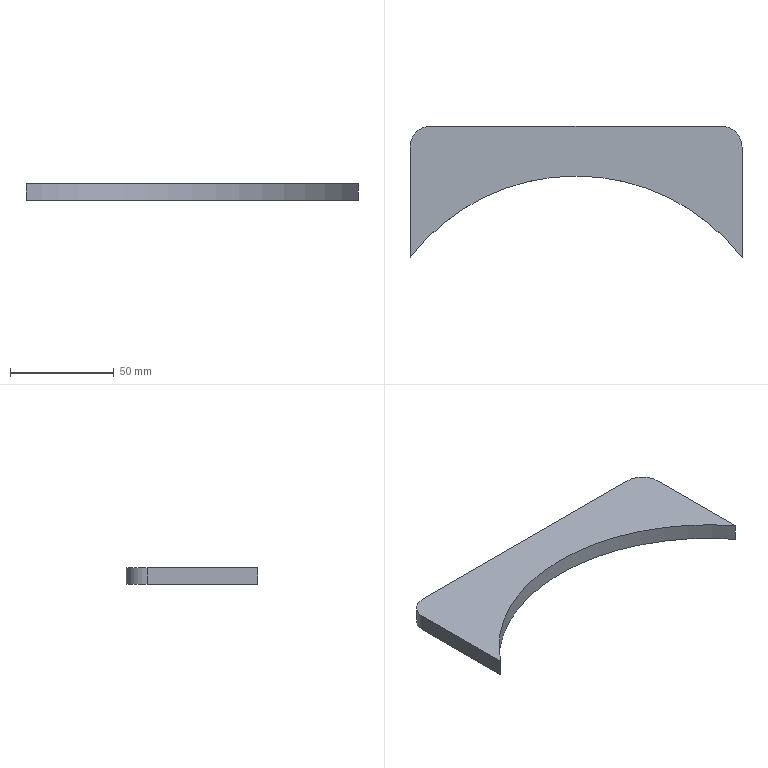Part | SolidWorks | features Extrusion 1, Fillet 1 | 1 solid | 8 faces | box 160 x 63.348 x 8 mm | volume 45593 mm3 | plane 5 | cylinder 3 | commonest cylinder face diameters 20 x2 202 x1
STEP:
#1=CARTESIAN_POINT('',(80.,61.652,0.));
#2=VERTEX_POINT('',#1);
#3=CARTESIAN_POINT('',(80.,115.,0.));
#4=VERTEX_POINT('',#3);
#5=CARTESIAN_POINT('',(80.,125.,0.));
#6=DIRECTION('',(0.,1.,0.));
#7=VECTOR('',#6,1000.);
#8=LINE('',#5,#7);
#9=EDGE_CURVE('',#2,#4,#8,.T.);
#10=ORIENTED_EDGE('',*,*,#9,.T.);
#11=CARTESIAN_POINT('',(80.,115.,8.));
#12=VERTEX_POINT('',#11);
#13=CARTESIAN_POINT('',(80.,115.,8.));
#14=DIRECTION('',(0.,0.,1.));
#15=VECTOR('',#14,1000.);
#16=LINE('',#13,#15);
#17=EDGE_CURVE('',#4,#12,#16,.T.);
#18=ORIENTED_EDGE('',*,*,#17,.T.);
#19=CARTESIAN_POINT('',(80.,61.652,8.));
#20=VERTEX_POINT('',#19);
#21=CARTESIAN_POINT('',(80.,125.,8.));
#22=DIRECTION('',(0.,1.,0.));
#23=VECTOR('',#22,1000.);
#24=LINE('',#21,#23);
#25=EDGE_CURVE('',#20,#12,#24,.T.);
#26=ORIENTED_EDGE('',*,*,#25,.F.);
#27=CARTESIAN_POINT('',(80.,61.652,8.));
#28=DIRECTION('',(0.,0.,-1.));
#29=VECTOR('',#28,1000.);
#30=LINE('',#27,#29);
#31=EDGE_CURVE('',#20,#2,#30,.T.);
#32=ORIENTED_EDGE('',*,*,#31,.T.);
#33=EDGE_LOOP('',(#10,#18,#26,#32));
#34=FACE_OUTER_BOUND('',#33,.T.);
#35=CARTESIAN_POINT('',(80.,125.,8.));
#36=DIRECTION('',(-1.,0.,0.));
#37=DIRECTION('',(0.,-1.,0.));
#38=AXIS2_PLACEMENT_3D('',#35,#36,#37);
#39=PLANE('',#38);
#40=ADVANCED_FACE('',(#34),#39,.F.);
#41=CARTESIAN_POINT('',(70.,125.,0.));
#42=VERTEX_POINT('',#41);
#43=CARTESIAN_POINT('',(-70.,125.,0.));
#44=VERTEX_POINT('',#43);
#45=CARTESIAN_POINT('',(80.,125.,0.));
#46=DIRECTION('',(-1.,0.,0.));
#47=VECTOR('',#46,1000.);
#48=LINE('',#45,#47);
#49=EDGE_CURVE('',#42,#44,#48,.T.);
#50=ORIENTED_EDGE('',*,*,#49,.T.);
#51=CARTESIAN_POINT('',(-70.,125.,8.));
#52=VERTEX_POINT('',#51);
#53=CARTESIAN_POINT('',(-70.,125.,8.));
#54=DIRECTION('',(0.,0.,1.));
#55=VECTOR('',#54,1000.);
#56=LINE('',#53,#55);
#57=EDGE_CURVE('',#44,#52,#56,.T.);
#58=ORIENTED_EDGE('',*,*,#57,.T.);
#59=CARTESIAN_POINT('',(70.,125.,8.));
#60=VERTEX_POINT('',#59);
#61=CARTESIAN_POINT('',(80.,125.,8.));
#62=DIRECTION('',(-1.,0.,0.));
#63=VECTOR('',#62,1000.);
#64=LINE('',#61,#63);
#65=EDGE_CURVE('',#60,#52,#64,.T.);
#66=ORIENTED_EDGE('',*,*,#65,.F.);
#67=CARTESIAN_POINT('',(70.,125.,8.));
#68=DIRECTION('',(0.,0.,-1.));
#69=VECTOR('',#68,1000.);
#70=LINE('',#67,#69);
#71=EDGE_CURVE('',#60,#42,#70,.T.);
#72=ORIENTED_EDGE('',*,*,#71,.T.);
#73=EDGE_LOOP('',(#50,#58,#66,#72));
#74=FACE_OUTER_BOUND('',#73,.T.);
#75=CARTESIAN_POINT('',(80.,125.,8.));
#76=DIRECTION('',(0.,-1.,0.));
#77=DIRECTION('',(0.,0.,-1.));
#78=AXIS2_PLACEMENT_3D('',#75,#76,#77);
#79=PLANE('',#78);
#80=ADVANCED_FACE('',(#74),#79,.F.);
#81=CARTESIAN_POINT('',(-80.,115.,8.));
#82=VERTEX_POINT('',#81);
#83=CARTESIAN_POINT('',(-80.,61.652,8.));
#84=VERTEX_POINT('',#83);
#85=CARTESIAN_POINT('',(-80.,125.,8.));
#86=DIRECTION('',(0.,-1.,0.));
#87=VECTOR('',#86,1000.);
#88=LINE('',#85,#87);
#89=EDGE_CURVE('',#82,#84,#88,.T.);
#90=ORIENTED_EDGE('',*,*,#89,.F.);
#91=CARTESIAN_POINT('',(-80.,115.,0.));
#92=VERTEX_POINT('',#91);
#93=CARTESIAN_POINT('',(-80.,115.,8.));
#94=DIRECTION('',(0.,0.,-1.));
#95=VECTOR('',#94,1000.);
#96=LINE('',#93,#95);
#97=EDGE_CURVE('',#82,#92,#96,.T.);
#98=ORIENTED_EDGE('',*,*,#97,.T.);
#99=CARTESIAN_POINT('',(-80.,61.652,0.));
#100=VERTEX_POINT('',#99);
#101=CARTESIAN_POINT('',(-80.,125.,0.));
#102=DIRECTION('',(0.,-1.,0.));
#103=VECTOR('',#102,1000.);
#104=LINE('',#101,#103);
#105=EDGE_CURVE('',#92,#100,#104,.T.);
#106=ORIENTED_EDGE('',*,*,#105,.T.);
#107=CARTESIAN_POINT('',(-80.,61.652,8.));
#108=DIRECTION('',(0.,0.,-1.));
#109=VECTOR('',#108,1000.);
#110=LINE('',#107,#109);
#111=EDGE_CURVE('',#84,#100,#110,.T.);
#112=ORIENTED_EDGE('',*,*,#111,.F.);
#113=EDGE_LOOP('',(#90,#98,#106,#112));
#114=FACE_OUTER_BOUND('',#113,.T.);
#115=CARTESIAN_POINT('',(-80.,125.,8.));
#116=DIRECTION('',(1.,0.,0.));
#117=DIRECTION('',(0.,1.,0.));
#118=AXIS2_PLACEMENT_3D('',#115,#116,#117);
#119=PLANE('',#118);
#120=ADVANCED_FACE('',(#114),#119,.F.);
#121=CARTESIAN_POINT('',(0.,0.,0.));
#122=DIRECTION('',(0.,0.,-1.));
#123=DIRECTION('',(1.,0.,0.));
#124=AXIS2_PLACEMENT_3D('',#121,#122,#123);
#125=CIRCLE('',#124,101.);
#126=EDGE_CURVE('',#100,#2,#125,.T.);
#127=ORIENTED_EDGE('',*,*,#126,.T.);
#128=ORIENTED_EDGE('',*,*,#31,.F.);
#129=CARTESIAN_POINT('',(0.,0.,8.));
#130=DIRECTION('',(0.,0.,-1.));
#131=DIRECTION('',(1.,0.,0.));
#132=AXIS2_PLACEMENT_3D('',#129,#130,#131);
#133=CIRCLE('',#132,101.);
#134=EDGE_CURVE('',#84,#20,#133,.T.);
#135=ORIENTED_EDGE('',*,*,#134,.F.);
#136=ORIENTED_EDGE('',*,*,#111,.T.);
#137=EDGE_LOOP('',(#127,#128,#135,#136));
#138=FACE_OUTER_BOUND('',#137,.T.);
#139=CARTESIAN_POINT('',(0.,0.,8.));
#140=DIRECTION('',(0.,0.,-1.));
#141=DIRECTION('',(-1.,0.,0.));
#142=AXIS2_PLACEMENT_3D('',#139,#140,#141);
#143=CYLINDRICAL_SURFACE('',#142,101.);
#144=ADVANCED_FACE('',(#138),#143,.F.);
#145=ORIENTED_EDGE('',*,*,#65,.T.);
#146=CARTESIAN_POINT('',(-70.,115.,8.));
#147=DIRECTION('',(0.,0.,1.));
#148=DIRECTION('',(1.,0.,0.));
#149=AXIS2_PLACEMENT_3D('',#146,#147,#148);
#150=CIRCLE('',#149,10.);
#151=EDGE_CURVE('',#52,#82,#150,.T.);
#152=ORIENTED_EDGE('',*,*,#151,.T.);
#153=ORIENTED_EDGE('',*,*,#89,.T.);
#154=ORIENTED_EDGE('',*,*,#134,.T.);
#155=ORIENTED_EDGE('',*,*,#25,.T.);
#156=CARTESIAN_POINT('',(70.,115.,8.));
#157=DIRECTION('',(0.,0.,1.));
#158=DIRECTION('',(1.,0.,0.));
#159=AXIS2_PLACEMENT_3D('',#156,#157,#158);
#160=CIRCLE('',#159,10.);
#161=EDGE_CURVE('',#12,#60,#160,.T.);
#162=ORIENTED_EDGE('',*,*,#161,.T.);
#163=EDGE_LOOP('',(#145,#152,#153,#154,#155,#162));
#164=FACE_OUTER_BOUND('',#163,.T.);
#165=CARTESIAN_POINT('',(0.,0.,8.));
#166=DIRECTION('',(0.,0.,1.));
#167=DIRECTION('',(1.,0.,0.));
#168=AXIS2_PLACEMENT_3D('',#165,#166,#167);
#169=PLANE('',#168);
#170=ADVANCED_FACE('',(#164),#169,.T.);
#171=ORIENTED_EDGE('',*,*,#105,.F.);
#172=CARTESIAN_POINT('',(-70.,115.,0.));
#173=DIRECTION('',(0.,0.,-1.));
#174=DIRECTION('',(1.,0.,0.));
#175=AXIS2_PLACEMENT_3D('',#172,#173,#174);
#176=CIRCLE('',#175,10.);
#177=EDGE_CURVE('',#92,#44,#176,.T.);
#178=ORIENTED_EDGE('',*,*,#177,.T.);
#179=ORIENTED_EDGE('',*,*,#49,.F.);
#180=CARTESIAN_POINT('',(70.,115.,0.));
#181=DIRECTION('',(0.,0.,-1.));
#182=DIRECTION('',(1.,0.,0.));
#183=AXIS2_PLACEMENT_3D('',#180,#181,#182);
#184=CIRCLE('',#183,10.);
#185=EDGE_CURVE('',#42,#4,#184,.T.);
#186=ORIENTED_EDGE('',*,*,#185,.T.);
#187=ORIENTED_EDGE('',*,*,#9,.F.);
#188=ORIENTED_EDGE('',*,*,#126,.F.);
#189=EDGE_LOOP('',(#171,#178,#179,#186,#187,#188));
#190=FACE_OUTER_BOUND('',#189,.T.);
#191=CARTESIAN_POINT('',(0.,0.,0.));
#192=DIRECTION('',(0.,0.,1.));
#193=DIRECTION('',(1.,0.,0.));
#194=AXIS2_PLACEMENT_3D('',#191,#192,#193);
#195=PLANE('',#194);
#196=ADVANCED_FACE('',(#190),#195,.F.);
#197=ORIENTED_EDGE('',*,*,#151,.F.);
#198=ORIENTED_EDGE('',*,*,#57,.F.);
#199=ORIENTED_EDGE('',*,*,#177,.F.);
#200=ORIENTED_EDGE('',*,*,#97,.F.);
#201=EDGE_LOOP('',(#197,#198,#199,#200));
#202=FACE_OUTER_BOUND('',#201,.T.);
#203=CARTESIAN_POINT('',(-70.,115.,8.));
#204=DIRECTION('',(0.,0.,-1.));
#205=DIRECTION('',(-1.,0.,0.));
#206=AXIS2_PLACEMENT_3D('',#203,#204,#205);
#207=CYLINDRICAL_SURFACE('',#206,10.);
#208=ADVANCED_FACE('',(#202),#207,.T.);
#209=ORIENTED_EDGE('',*,*,#161,.F.);
#210=ORIENTED_EDGE('',*,*,#17,.F.);
#211=ORIENTED_EDGE('',*,*,#185,.F.);
#212=ORIENTED_EDGE('',*,*,#71,.F.);
#213=EDGE_LOOP('',(#209,#210,#211,#212));
#214=FACE_OUTER_BOUND('',#213,.T.);
#215=CARTESIAN_POINT('',(70.,115.,8.));
#216=DIRECTION('',(0.,0.,-1.));
#217=DIRECTION('',(-1.,0.,0.));
#218=AXIS2_PLACEMENT_3D('',#215,#216,#217);
#219=CYLINDRICAL_SURFACE('',#218,10.);
#220=ADVANCED_FACE('',(#214),#219,.T.);
#221=CLOSED_SHELL('',(#40,#80,#120,#144,#170,#196,#208,#220));
#222=MANIFOLD_SOLID_BREP('',#221);
#223=CARTESIAN_POINT('',(0.,0.,0.));
#224=DIRECTION('',(0.,0.,1.));
#225=DIRECTION('',(1.,0.,0.));
#226=AXIS2_PLACEMENT_3D('',#223,#224,#225);
#227=(LENGTH_UNIT()NAMED_UNIT(*)SI_UNIT(.MILLI.,.METRE.));
#228=UNCERTAINTY_MEASURE_WITH_UNIT(LENGTH_MEASURE(0.00001),#227,'','');
#229=(NAMED_UNIT(*)PLANE_ANGLE_UNIT()SI_UNIT($,.RADIAN.));
#230=(NAMED_UNIT(*)SI_UNIT($,.STERADIAN.)SOLID_ANGLE_UNIT());
#231=(GEOMETRIC_REPRESENTATION_CONTEXT(3)GLOBAL_UNCERTAINTY_ASSIGNED_CONTEXT((#228))GLOBAL_UNIT_ASSIGNED_CONTEXT((#227,#229,#230))REPRESENTATION_CONTEXT('',''));
#232=ADVANCED_BREP_SHAPE_REPRESENTATION('',(#222,#226),#231);